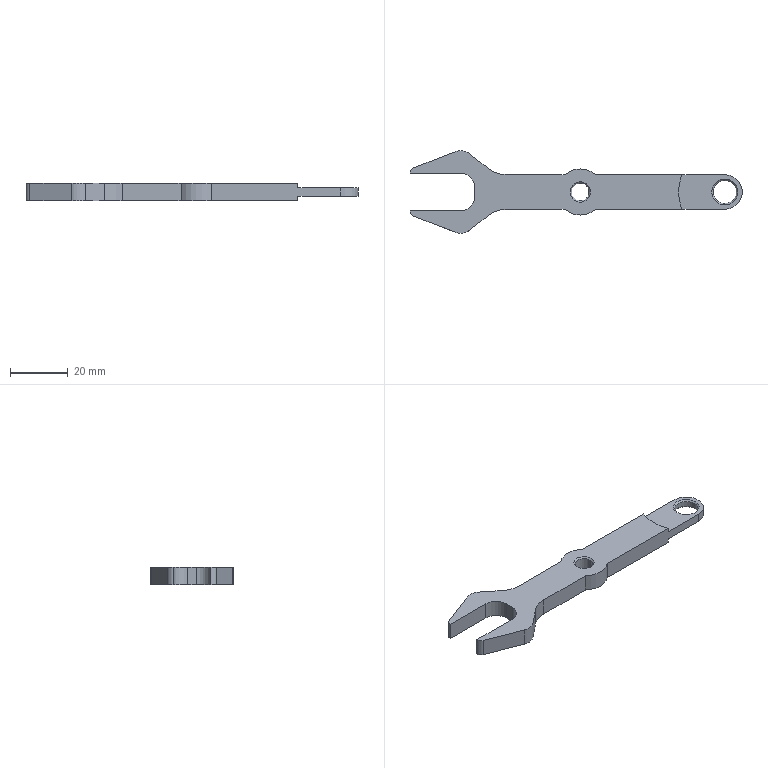Part | SolidWorks | features ICE 2, Chamfer 1, Extrusion 1, Fillet 1, MirrorPattern 1 | 1 solid | 41 faces | box 114.951 x 28.607 x 6 mm | volume 7418 mm3 | cylinder 18 | plane 15 | cone 8 | commonest cylinder face diameters 10 x4 32 x3 4 x2 6 x2 8 x2 16 x2
STEP:
#1=CARTESIAN_POINT('',(3.,0.,-2.5));
#2=VERTEX_POINT('',#1);
#3=CARTESIAN_POINT('',(-3.,0.,-2.5));
#4=VERTEX_POINT('',#3);
#5=CARTESIAN_POINT('',(0.,0.,-2.5));
#6=DIRECTION('',(0.,0.,-1.));
#7=DIRECTION('',(-1.,0.,0.));
#8=AXIS2_PLACEMENT_3D('',#5,#6,#7);
#9=CIRCLE('',#8,3.);
#10=EDGE_CURVE('',#2,#4,#9,.T.);
#11=ORIENTED_EDGE('',*,*,#10,.F.);
#12=CARTESIAN_POINT('',(3.5,0.,-3.));
#13=VERTEX_POINT('',#12);
#14=CARTESIAN_POINT('',(3.5,0.,-3.));
#15=DIRECTION('',(0.7071,0.,-0.7071));
#16=VECTOR('',#15,1000.);
#17=LINE('',#14,#16);
#18=EDGE_CURVE('',#2,#13,#17,.T.);
#19=ORIENTED_EDGE('',*,*,#18,.T.);
#20=CARTESIAN_POINT('',(-3.5,0.,-3.));
#21=VERTEX_POINT('',#20);
#22=CARTESIAN_POINT('',(0.,0.,-3.));
#23=DIRECTION('',(0.,0.,1.));
#24=DIRECTION('',(-1.,0.,0.));
#25=AXIS2_PLACEMENT_3D('',#22,#23,#24);
#26=CIRCLE('',#25,3.5);
#27=EDGE_CURVE('',#21,#13,#26,.T.);
#28=ORIENTED_EDGE('',*,*,#27,.F.);
#29=CARTESIAN_POINT('',(-3.5,0.,-3.));
#30=DIRECTION('',(-0.7071,0.,-0.7071));
#31=VECTOR('',#30,1000.);
#32=LINE('',#29,#31);
#33=EDGE_CURVE('',#4,#21,#32,.T.);
#34=ORIENTED_EDGE('',*,*,#33,.F.);
#35=EDGE_LOOP('',(#11,#19,#28,#34));
#36=FACE_OUTER_BOUND('',#35,.T.);
#37=CARTESIAN_POINT('',(0.,0.,-3.));
#38=DIRECTION('',(0.,0.,-1.));
#39=DIRECTION('',(-1.,0.,0.));
#40=AXIS2_PLACEMENT_3D('',#37,#38,#39);
#41=CONICAL_SURFACE('',#40,3.5,0.7854);
#42=ADVANCED_FACE('',(#36),#41,.F.);
#43=CARTESIAN_POINT('',(-3.,0.,2.5));
#44=VERTEX_POINT('',#43);
#45=CARTESIAN_POINT('',(3.,0.,2.5));
#46=VERTEX_POINT('',#45);
#47=CARTESIAN_POINT('',(0.,0.,2.5));
#48=DIRECTION('',(0.,0.,1.));
#49=DIRECTION('',(-1.,0.,0.));
#50=AXIS2_PLACEMENT_3D('',#47,#48,#49);
#51=CIRCLE('',#50,3.);
#52=EDGE_CURVE('',#44,#46,#51,.T.);
#53=ORIENTED_EDGE('',*,*,#52,.F.);
#54=CARTESIAN_POINT('',(-3.5,0.,3.));
#55=VERTEX_POINT('',#54);
#56=CARTESIAN_POINT('',(-3.,0.,2.5));
#57=DIRECTION('',(-0.7071,0.,0.7071));
#58=VECTOR('',#57,1000.);
#59=LINE('',#56,#58);
#60=EDGE_CURVE('',#44,#55,#59,.T.);
#61=ORIENTED_EDGE('',*,*,#60,.T.);
#62=CARTESIAN_POINT('',(3.5,0.,3.));
#63=VERTEX_POINT('',#62);
#64=CARTESIAN_POINT('',(0.,0.,3.));
#65=DIRECTION('',(0.,0.,-1.));
#66=DIRECTION('',(-1.,0.,0.));
#67=AXIS2_PLACEMENT_3D('',#64,#65,#66);
#68=CIRCLE('',#67,3.5);
#69=EDGE_CURVE('',#63,#55,#68,.T.);
#70=ORIENTED_EDGE('',*,*,#69,.F.);
#71=CARTESIAN_POINT('',(3.,0.,2.5));
#72=DIRECTION('',(0.7071,0.,0.7071));
#73=VECTOR('',#72,1000.);
#74=LINE('',#71,#73);
#75=EDGE_CURVE('',#46,#63,#74,.T.);
#76=ORIENTED_EDGE('',*,*,#75,.F.);
#77=EDGE_LOOP('',(#53,#61,#70,#76));
#78=FACE_OUTER_BOUND('',#77,.T.);
#79=CARTESIAN_POINT('',(0.,0.,2.5));
#80=DIRECTION('',(0.,0.,1.));
#81=DIRECTION('',(1.,0.,0.));
#82=AXIS2_PLACEMENT_3D('',#79,#80,#81);
#83=CONICAL_SURFACE('',#82,3.,0.7854);
#84=ADVANCED_FACE('',(#78),#83,.F.);
#85=CARTESIAN_POINT('',(46.,0.,1.));
#86=VERTEX_POINT('',#85);
#87=CARTESIAN_POINT('',(54.,0.,1.));
#88=VERTEX_POINT('',#87);
#89=CARTESIAN_POINT('',(50.,0.,1.));
#90=DIRECTION('',(0.,0.,1.));
#91=DIRECTION('',(1.,0.,0.));
#92=AXIS2_PLACEMENT_3D('',#89,#90,#91);
#93=CIRCLE('',#92,4.);
#94=EDGE_CURVE('',#86,#88,#93,.T.);
#95=ORIENTED_EDGE('',*,*,#94,.F.);
#96=CARTESIAN_POINT('',(45.5,0.,1.5));
#97=VERTEX_POINT('',#96);
#98=CARTESIAN_POINT('',(46.,0.,1.));
#99=DIRECTION('',(-0.7071,0.,0.7071));
#100=VECTOR('',#99,1000.);
#101=LINE('',#98,#100);
#102=EDGE_CURVE('',#86,#97,#101,.T.);
#103=ORIENTED_EDGE('',*,*,#102,.T.);
#104=CARTESIAN_POINT('',(54.5,0.,1.5));
#105=VERTEX_POINT('',#104);
#106=CARTESIAN_POINT('',(50.,0.,1.5));
#107=DIRECTION('',(0.,0.,-1.));
#108=DIRECTION('',(1.,0.,0.));
#109=AXIS2_PLACEMENT_3D('',#106,#107,#108);
#110=CIRCLE('',#109,4.5);
#111=EDGE_CURVE('',#105,#97,#110,.T.);
#112=ORIENTED_EDGE('',*,*,#111,.F.);
#113=CARTESIAN_POINT('',(54.,0.,1.));
#114=DIRECTION('',(0.7071,0.,0.7071));
#115=VECTOR('',#114,1000.);
#116=LINE('',#113,#115);
#117=EDGE_CURVE('',#88,#105,#116,.T.);
#118=ORIENTED_EDGE('',*,*,#117,.F.);
#119=EDGE_LOOP('',(#95,#103,#112,#118));
#120=FACE_OUTER_BOUND('',#119,.T.);
#121=CARTESIAN_POINT('',(50.,0.,1.));
#122=DIRECTION('',(0.,0.,1.));
#123=DIRECTION('',(1.,0.,0.));
#124=AXIS2_PLACEMENT_3D('',#121,#122,#123);
#125=CONICAL_SURFACE('',#124,4.,0.7854);
#126=ADVANCED_FACE('',(#120),#125,.F.);
#127=CARTESIAN_POINT('',(54.,0.,-1.));
#128=VERTEX_POINT('',#127);
#129=CARTESIAN_POINT('',(46.,0.,-1.));
#130=VERTEX_POINT('',#129);
#131=CARTESIAN_POINT('',(50.,0.,-1.));
#132=DIRECTION('',(0.,0.,-1.));
#133=DIRECTION('',(-1.,0.,0.));
#134=AXIS2_PLACEMENT_3D('',#131,#132,#133);
#135=CIRCLE('',#134,4.);
#136=EDGE_CURVE('',#128,#130,#135,.T.);
#137=ORIENTED_EDGE('',*,*,#136,.F.);
#138=CARTESIAN_POINT('',(54.5,0.,-1.5));
#139=VERTEX_POINT('',#138);
#140=CARTESIAN_POINT('',(54.,0.,-1.));
#141=DIRECTION('',(0.7071,0.,-0.7071));
#142=VECTOR('',#141,1000.);
#143=LINE('',#140,#142);
#144=EDGE_CURVE('',#128,#139,#143,.T.);
#145=ORIENTED_EDGE('',*,*,#144,.T.);
#146=CARTESIAN_POINT('',(45.5,0.,-1.5));
#147=VERTEX_POINT('',#146);
#148=CARTESIAN_POINT('',(50.,0.,-1.5));
#149=DIRECTION('',(0.,0.,1.));
#150=DIRECTION('',(-1.,0.,0.));
#151=AXIS2_PLACEMENT_3D('',#148,#149,#150);
#152=CIRCLE('',#151,4.5);
#153=EDGE_CURVE('',#147,#139,#152,.T.);
#154=ORIENTED_EDGE('',*,*,#153,.F.);
#155=CARTESIAN_POINT('',(46.,0.,-1.));
#156=DIRECTION('',(-0.7071,0.,-0.7071));
#157=VECTOR('',#156,1000.);
#158=LINE('',#155,#157);
#159=EDGE_CURVE('',#130,#147,#158,.T.);
#160=ORIENTED_EDGE('',*,*,#159,.F.);
#161=EDGE_LOOP('',(#137,#145,#154,#160));
#162=FACE_OUTER_BOUND('',#161,.T.);
#163=CARTESIAN_POINT('',(50.,0.,-1.));
#164=DIRECTION('',(0.,0.,-1.));
#165=DIRECTION('',(-1.,0.,0.));
#166=AXIS2_PLACEMENT_3D('',#163,#164,#165);
#167=CONICAL_SURFACE('',#166,4.,0.7854);
#168=ADVANCED_FACE('',(#162),#167,.F.);
#169=ORIENTED_EDGE('',*,*,#10,.T.);
#170=CARTESIAN_POINT('',(-3.,0.,-3.));
#171=DIRECTION('',(0.,0.,1.));
#172=VECTOR('',#171,1000.);
#173=LINE('',#170,#172);
#174=EDGE_CURVE('',#4,#44,#173,.T.);
#175=ORIENTED_EDGE('',*,*,#174,.T.);
#176=ORIENTED_EDGE('',*,*,#52,.T.);
#177=CARTESIAN_POINT('',(3.,0.,-3.));
#178=DIRECTION('',(0.,0.,1.));
#179=VECTOR('',#178,1000.);
#180=LINE('',#177,#179);
#181=EDGE_CURVE('',#2,#46,#180,.T.);
#182=ORIENTED_EDGE('',*,*,#181,.F.);
#183=EDGE_LOOP('',(#169,#175,#176,#182));
#184=FACE_OUTER_BOUND('',#183,.T.);
#185=CARTESIAN_POINT('',(0.,0.,-3.));
#186=DIRECTION('',(0.,0.,1.));
#187=DIRECTION('',(1.,0.,0.));
#188=AXIS2_PLACEMENT_3D('',#185,#186,#187);
#189=CYLINDRICAL_SURFACE('',#188,3.);
#190=ADVANCED_FACE('',(#184),#189,.F.);
#191=ORIENTED_EDGE('',*,*,#136,.T.);
#192=CARTESIAN_POINT('',(46.,0.,-3.));
#193=DIRECTION('',(0.,0.,1.));
#194=VECTOR('',#193,1000.);
#195=LINE('',#192,#194);
#196=EDGE_CURVE('',#130,#86,#195,.T.);
#197=ORIENTED_EDGE('',*,*,#196,.T.);
#198=ORIENTED_EDGE('',*,*,#94,.T.);
#199=CARTESIAN_POINT('',(54.,0.,-3.));
#200=DIRECTION('',(0.,0.,1.));
#201=VECTOR('',#200,1000.);
#202=LINE('',#199,#201);
#203=EDGE_CURVE('',#128,#88,#202,.T.);
#204=ORIENTED_EDGE('',*,*,#203,.F.);
#205=EDGE_LOOP('',(#191,#197,#198,#204));
#206=FACE_OUTER_BOUND('',#205,.T.);
#207=CARTESIAN_POINT('',(50.,0.,-3.));
#208=DIRECTION('',(0.,0.,1.));
#209=DIRECTION('',(1.,0.,0.));
#210=AXIS2_PLACEMENT_3D('',#207,#208,#209);
#211=CYLINDRICAL_SURFACE('',#210,4.);
#212=ADVANCED_FACE('',(#206),#211,.F.);
#213=CARTESIAN_POINT('',(35.168,6.,-1.5));
#214=VERTEX_POINT('',#213);
#215=CARTESIAN_POINT('',(34.,0.,-1.5));
#216=VERTEX_POINT('',#215);
#217=CARTESIAN_POINT('',(50.,0.,-1.5));
#218=DIRECTION('',(0.,0.,1.));
#219=DIRECTION('',(1.,0.,0.));
#220=AXIS2_PLACEMENT_3D('',#217,#218,#219);
#221=CIRCLE('',#220,16.);
#222=EDGE_CURVE('',#214,#216,#221,.T.);
#223=ORIENTED_EDGE('',*,*,#222,.T.);
#224=CARTESIAN_POINT('',(34.,0.,-3.));
#225=VERTEX_POINT('',#224);
#226=CARTESIAN_POINT('',(34.,0.,-1.5));
#227=DIRECTION('',(0.,0.,-1.));
#228=VECTOR('',#227,1000.);
#229=LINE('',#226,#228);
#230=EDGE_CURVE('',#216,#225,#229,.T.);
#231=ORIENTED_EDGE('',*,*,#230,.T.);
#232=CARTESIAN_POINT('',(35.168,6.,-3.));
#233=VERTEX_POINT('',#232);
#234=CARTESIAN_POINT('',(50.,0.,-3.));
#235=DIRECTION('',(0.,0.,1.));
#236=DIRECTION('',(1.,0.,0.));
#237=AXIS2_PLACEMENT_3D('',#234,#235,#236);
#238=CIRCLE('',#237,16.);
#239=EDGE_CURVE('',#233,#225,#238,.T.);
#240=ORIENTED_EDGE('',*,*,#239,.F.);
#241=CARTESIAN_POINT('',(35.168,6.,-1.5));
#242=DIRECTION('',(0.,0.,1.));
#243=VECTOR('',#242,1000.);
#244=LINE('',#241,#243);
#245=EDGE_CURVE('',#233,#214,#244,.T.);
#246=ORIENTED_EDGE('',*,*,#245,.T.);
#247=EDGE_LOOP('',(#223,#231,#240,#246));
#248=FACE_OUTER_BOUND('',#247,.T.);
#249=CARTESIAN_POINT('',(50.,0.,-1.5));
#250=DIRECTION('',(0.,0.,-1.));
#251=DIRECTION('',(-1.,0.,0.));
#252=AXIS2_PLACEMENT_3D('',#249,#250,#251);
#253=CYLINDRICAL_SURFACE('',#252,16.);
#254=ADVANCED_FACE('',(#248),#253,.F.);
#255=CARTESIAN_POINT('',(50.,6.,-1.5));
#256=VERTEX_POINT('',#255);
#257=CARTESIAN_POINT('',(50.,-6.,-1.5));
#258=VERTEX_POINT('',#257);
#259=CARTESIAN_POINT('',(50.,0.,-1.5));
#260=DIRECTION('',(0.,0.,-1.));
#261=DIRECTION('',(-1.,0.,0.));
#262=AXIS2_PLACEMENT_3D('',#259,#260,#261);
#263=CIRCLE('',#262,6.);
#264=EDGE_CURVE('',#256,#258,#263,.T.);
#265=ORIENTED_EDGE('',*,*,#264,.F.);
#266=CARTESIAN_POINT('',(50.,6.,1.5));
#267=VERTEX_POINT('',#266);
#268=CARTESIAN_POINT('',(50.,6.,3.));
#269=DIRECTION('',(0.,0.,-1.));
#270=VECTOR('',#269,1000.);
#271=LINE('',#268,#270);
#272=EDGE_CURVE('',#267,#256,#271,.T.);
#273=ORIENTED_EDGE('',*,*,#272,.F.);
#274=CARTESIAN_POINT('',(50.,-6.,1.5));
#275=VERTEX_POINT('',#274);
#276=CARTESIAN_POINT('',(50.,0.,1.5));
#277=DIRECTION('',(0.,0.,1.));
#278=DIRECTION('',(1.,0.,0.));
#279=AXIS2_PLACEMENT_3D('',#276,#277,#278);
#280=CIRCLE('',#279,6.);
#281=EDGE_CURVE('',#275,#267,#280,.T.);
#282=ORIENTED_EDGE('',*,*,#281,.F.);
#283=CARTESIAN_POINT('',(50.,-6.,3.));
#284=DIRECTION('',(0.,0.,-1.));
#285=VECTOR('',#284,1000.);
#286=LINE('',#283,#285);
#287=EDGE_CURVE('',#275,#258,#286,.T.);
#288=ORIENTED_EDGE('',*,*,#287,.T.);
#289=EDGE_LOOP('',(#265,#273,#282,#288));
#290=FACE_OUTER_BOUND('',#289,.T.);
#291=CARTESIAN_POINT('',(50.,0.,3.));
#292=DIRECTION('',(0.,0.,-1.));
#293=DIRECTION('',(-1.,0.,0.));
#294=AXIS2_PLACEMENT_3D('',#291,#292,#293);
#295=CYLINDRICAL_SURFACE('',#294,6.);
#296=ADVANCED_FACE('',(#290),#295,.T.);
#297=CARTESIAN_POINT('',(35.168,-6.,-1.5));
#298=VERTEX_POINT('',#297);
#299=CARTESIAN_POINT('',(35.168,-6.,-3.));
#300=VERTEX_POINT('',#299);
#301=CARTESIAN_POINT('',(35.168,-6.,-1.5));
#302=DIRECTION('',(0.,0.,-1.));
#303=VECTOR('',#302,1000.);
#304=LINE('',#301,#303);
#305=EDGE_CURVE('',#298,#300,#304,.T.);
#306=ORIENTED_EDGE('',*,*,#305,.F.);
#307=CARTESIAN_POINT('',(50.,-6.,-1.5));
#308=DIRECTION('',(-1.,0.,0.));
#309=VECTOR('',#308,1000.);
#310=LINE('',#307,#309);
#311=EDGE_CURVE('',#258,#298,#310,.T.);
#312=ORIENTED_EDGE('',*,*,#311,.F.);
#313=ORIENTED_EDGE('',*,*,#287,.F.);
#314=CARTESIAN_POINT('',(35.168,-6.,1.5));
#315=VERTEX_POINT('',#314);
#316=CARTESIAN_POINT('',(50.,-6.,1.5));
#317=DIRECTION('',(1.,0.,0.));
#318=VECTOR('',#317,1000.);
#319=LINE('',#316,#318);
#320=EDGE_CURVE('',#315,#275,#319,.T.);
#321=ORIENTED_EDGE('',*,*,#320,.F.);
#322=CARTESIAN_POINT('',(35.168,-6.,3.));
#323=VERTEX_POINT('',#322);
#324=CARTESIAN_POINT('',(35.168,-6.,1.5));
#325=DIRECTION('',(0.,0.,1.));
#326=VECTOR('',#325,1000.);
#327=LINE('',#324,#326);
#328=EDGE_CURVE('',#315,#323,#327,.T.);
#329=ORIENTED_EDGE('',*,*,#328,.T.);
#330=CARTESIAN_POINT('',(5.292,-6.,3.));
#331=VERTEX_POINT('',#330);
#332=CARTESIAN_POINT('',(50.,-6.,3.));
#333=DIRECTION('',(1.,0.,0.));
#334=VECTOR('',#333,1000.);
#335=LINE('',#332,#334);
#336=EDGE_CURVE('',#331,#323,#335,.T.);
#337=ORIENTED_EDGE('',*,*,#336,.F.);
#338=CARTESIAN_POINT('',(5.292,-6.,-3.));
#339=VERTEX_POINT('',#338);
#340=CARTESIAN_POINT('',(5.292,-6.,3.));
#341=DIRECTION('',(0.,0.,-1.));
#342=VECTOR('',#341,1000.);
#343=LINE('',#340,#342);
#344=EDGE_CURVE('',#331,#339,#343,.T.);
#345=ORIENTED_EDGE('',*,*,#344,.T.);
#346=CARTESIAN_POINT('',(50.,-6.,-3.));
#347=DIRECTION('',(1.,0.,0.));
#348=VECTOR('',#347,1000.);
#349=LINE('',#346,#348);
#350=EDGE_CURVE('',#339,#300,#349,.T.);
#351=ORIENTED_EDGE('',*,*,#350,.T.);
#352=EDGE_LOOP('',(#306,#312,#313,#321,#329,#337,#345,#351));
#353=FACE_OUTER_BOUND('',#352,.T.);
#354=CARTESIAN_POINT('',(50.,-6.,3.));
#355=DIRECTION('',(0.,1.,0.));
#356=DIRECTION('',(0.,0.,1.));
#357=AXIS2_PLACEMENT_3D('',#354,#355,#356);
#358=PLANE('',#357);
#359=ADVANCED_FACE('',(#353),#358,.F.);
#360=ORIENTED_EDGE('',*,*,#245,.F.);
#361=CARTESIAN_POINT('',(5.292,6.,-3.));
#362=VERTEX_POINT('',#361);
#363=CARTESIAN_POINT('',(50.,6.,-3.));
#364=DIRECTION('',(-1.,0.,0.));
#365=VECTOR('',#364,1000.);
#366=LINE('',#363,#365);
#367=EDGE_CURVE('',#233,#362,#366,.T.);
#368=ORIENTED_EDGE('',*,*,#367,.T.);
#369=CARTESIAN_POINT('',(5.292,6.,3.));
#370=VERTEX_POINT('',#369);
#371=CARTESIAN_POINT('',(5.292,6.,3.));
#372=DIRECTION('',(0.,0.,-1.));
#373=VECTOR('',#372,1000.);
#374=LINE('',#371,#373);
#375=EDGE_CURVE('',#370,#362,#374,.T.);
#376=ORIENTED_EDGE('',*,*,#375,.F.);
#377=CARTESIAN_POINT('',(35.168,6.,3.));
#378=VERTEX_POINT('',#377);
#379=CARTESIAN_POINT('',(50.,6.,3.));
#380=DIRECTION('',(-1.,0.,0.));
#381=VECTOR('',#380,1000.);
#382=LINE('',#379,#381);
#383=EDGE_CURVE('',#378,#370,#382,.T.);
#384=ORIENTED_EDGE('',*,*,#383,.F.);
#385=CARTESIAN_POINT('',(35.168,6.,1.5));
#386=VERTEX_POINT('',#385);
#387=CARTESIAN_POINT('',(35.168,6.,1.5));
#388=DIRECTION('',(0.,0.,-1.));
#389=VECTOR('',#388,1000.);
#390=LINE('',#387,#389);
#391=EDGE_CURVE('',#378,#386,#390,.T.);
#392=ORIENTED_EDGE('',*,*,#391,.T.);
#393=CARTESIAN_POINT('',(50.,6.,1.5));
#394=DIRECTION('',(-1.,0.,0.));
#395=VECTOR('',#394,1000.);
#396=LINE('',#393,#395);
#397=EDGE_CURVE('',#267,#386,#396,.T.);
#398=ORIENTED_EDGE('',*,*,#397,.F.);
#399=ORIENTED_EDGE('',*,*,#272,.T.);
#400=CARTESIAN_POINT('',(50.,6.,-1.5));
#401=DIRECTION('',(1.,0.,0.));
#402=VECTOR('',#401,1000.);
#403=LINE('',#400,#402);
#404=EDGE_CURVE('',#214,#256,#403,.T.);
#405=ORIENTED_EDGE('',*,*,#404,.F.);
#406=EDGE_LOOP('',(#360,#368,#376,#384,#392,#398,#399,#405));
#407=FACE_OUTER_BOUND('',#406,.T.);
#408=CARTESIAN_POINT('',(50.,6.,3.));
#409=DIRECTION('',(0.,-1.,0.));
#410=DIRECTION('',(0.,0.,-1.));
#411=AXIS2_PLACEMENT_3D('',#408,#409,#410);
#412=PLANE('',#411);
#413=ADVANCED_FACE('',(#407),#412,.F.);
#414=CARTESIAN_POINT('',(-43.172,-13.967,-3.));
#415=VERTEX_POINT('',#414);
#416=CARTESIAN_POINT('',(-38.258,-13.217,-3.));
#417=VERTEX_POINT('',#416);
#418=CARTESIAN_POINT('',(-41.37,-9.303,-3.));
#419=DIRECTION('',(0.,0.,1.));
#420=DIRECTION('',(-1.,0.,0.));
#421=AXIS2_PLACEMENT_3D('',#418,#419,#420);
#422=CIRCLE('',#421,5.);
#423=EDGE_CURVE('',#415,#417,#422,.T.);
#424=ORIENTED_EDGE('',*,*,#423,.T.);
#425=CARTESIAN_POINT('',(-38.258,-13.217,3.));
#426=VERTEX_POINT('',#425);
#427=CARTESIAN_POINT('',(-38.258,-13.217,3.));
#428=DIRECTION('',(0.,0.,-1.));
#429=VECTOR('',#428,1000.);
#430=LINE('',#427,#429);
#431=EDGE_CURVE('',#426,#417,#430,.T.);
#432=ORIENTED_EDGE('',*,*,#431,.F.);
#433=CARTESIAN_POINT('',(-43.172,-13.967,3.));
#434=VERTEX_POINT('',#433);
#435=CARTESIAN_POINT('',(-41.37,-9.303,3.));
#436=DIRECTION('',(0.,0.,1.));
#437=DIRECTION('',(-1.,0.,0.));
#438=AXIS2_PLACEMENT_3D('',#435,#436,#437);
#439=CIRCLE('',#438,5.);
#440=EDGE_CURVE('',#434,#426,#439,.T.);
#441=ORIENTED_EDGE('',*,*,#440,.F.);
#442=CARTESIAN_POINT('',(-43.172,-13.967,3.));
#443=DIRECTION('',(0.,0.,-1.));
#444=VECTOR('',#443,1000.);
#445=LINE('',#442,#444);
#446=EDGE_CURVE('',#434,#415,#445,.T.);
#447=ORIENTED_EDGE('',*,*,#446,.T.);
#448=EDGE_LOOP('',(#424,#432,#441,#447));
#449=FACE_OUTER_BOUND('',#448,.T.);
#450=CARTESIAN_POINT('',(-41.37,-9.303,3.));
#451=DIRECTION('',(0.,0.,-1.));
#452=DIRECTION('',(-1.,0.,0.));
#453=AXIS2_PLACEMENT_3D('',#450,#451,#452);
#454=CYLINDRICAL_SURFACE('',#453,5.);
#455=ADVANCED_FACE('',(#449),#454,.T.);
#456=CARTESIAN_POINT('',(-31.918,-8.174,-3.));
#457=VERTEX_POINT('',#456);
#458=CARTESIAN_POINT('',(-29.185,-6.,-3.));
#459=DIRECTION('',(0.7826,0.6225,0.));
#460=VECTOR('',#459,1000.);
#461=LINE('',#458,#460);
#462=EDGE_CURVE('',#417,#457,#461,.T.);
#463=ORIENTED_EDGE('',*,*,#462,.T.);
#464=CARTESIAN_POINT('',(-31.918,-8.174,3.));
#465=VERTEX_POINT('',#464);
#466=CARTESIAN_POINT('',(-31.918,-8.174,3.));
#467=DIRECTION('',(0.,0.,1.));
#468=VECTOR('',#467,1000.);
#469=LINE('',#466,#468);
#470=EDGE_CURVE('',#457,#465,#469,.T.);
#471=ORIENTED_EDGE('',*,*,#470,.T.);
#472=CARTESIAN_POINT('',(-29.185,-6.,3.));
#473=DIRECTION('',(0.7826,0.6225,0.));
#474=VECTOR('',#473,1000.);
#475=LINE('',#472,#474);
#476=EDGE_CURVE('',#426,#465,#475,.T.);
#477=ORIENTED_EDGE('',*,*,#476,.F.);
#478=ORIENTED_EDGE('',*,*,#431,.T.);
#479=EDGE_LOOP('',(#463,#471,#477,#478));
#480=FACE_OUTER_BOUND('',#479,.T.);
#481=CARTESIAN_POINT('',(-29.185,-6.,3.));
#482=DIRECTION('',(-0.6225,0.7826,0.));
#483=DIRECTION('',(-0.7826,-0.6225,0.));
#484=AXIS2_PLACEMENT_3D('',#481,#482,#483);
#485=PLANE('',#484);
#486=ADVANCED_FACE('',(#480),#485,.F.);
#487=CARTESIAN_POINT('',(-25.693,-6.,3.));
#488=VERTEX_POINT('',#487);
#489=CARTESIAN_POINT('',(-5.292,-6.,3.));
#490=VERTEX_POINT('',#489);
#491=CARTESIAN_POINT('',(-5.292,-6.,3.));
#492=DIRECTION('',(1.,0.,0.));
#493=VECTOR('',#492,1000.);
#494=LINE('',#491,#493);
#495=EDGE_CURVE('',#488,#490,#494,.T.);
#496=ORIENTED_EDGE('',*,*,#495,.F.);
#497=CARTESIAN_POINT('',(-25.693,-6.,-3.));
#498=VERTEX_POINT('',#497);
#499=CARTESIAN_POINT('',(-25.693,-6.,-3.));
#500=DIRECTION('',(0.,0.,-1.));
#501=VECTOR('',#500,1000.);
#502=LINE('',#499,#501);
#503=EDGE_CURVE('',#488,#498,#502,.T.);
#504=ORIENTED_EDGE('',*,*,#503,.T.);
#505=CARTESIAN_POINT('',(-5.292,-6.,-3.));
#506=VERTEX_POINT('',#505);
#507=CARTESIAN_POINT('',(-5.292,-6.,-3.));
#508=DIRECTION('',(1.,0.,0.));
#509=VECTOR('',#508,1000.);
#510=LINE('',#507,#509);
#511=EDGE_CURVE('',#498,#506,#510,.T.);
#512=ORIENTED_EDGE('',*,*,#511,.T.);
#513=CARTESIAN_POINT('',(-5.292,-6.,3.));
#514=DIRECTION('',(0.,0.,-1.));
#515=VECTOR('',#514,1000.);
#516=LINE('',#513,#515);
#517=EDGE_CURVE('',#490,#506,#516,.T.);
#518=ORIENTED_EDGE('',*,*,#517,.F.);
#519=EDGE_LOOP('',(#496,#504,#512,#518));
#520=FACE_OUTER_BOUND('',#519,.T.);
#521=CARTESIAN_POINT('',(-5.292,-6.,3.));
#522=DIRECTION('',(0.,1.,0.));
#523=DIRECTION('',(-1.,0.,0.));
#524=AXIS2_PLACEMENT_3D('',#521,#522,#523);
#525=PLANE('',#524);
#526=ADVANCED_FACE('',(#520),#525,.F.);
#527=CARTESIAN_POINT('',(0.,0.,-3.));
#528=DIRECTION('',(0.,0.,1.));
#529=DIRECTION('',(-1.,0.,0.));
#530=AXIS2_PLACEMENT_3D('',#527,#528,#529);
#531=CIRCLE('',#530,8.);
#532=EDGE_CURVE('',#506,#339,#531,.T.);
#533=ORIENTED_EDGE('',*,*,#532,.T.);
#534=ORIENTED_EDGE('',*,*,#344,.F.);
#535=CARTESIAN_POINT('',(0.,0.,3.));
#536=DIRECTION('',(0.,0.,1.));
#537=DIRECTION('',(-1.,0.,0.));
#538=AXIS2_PLACEMENT_3D('',#535,#536,#537);
#539=CIRCLE('',#538,8.);
#540=EDGE_CURVE('',#490,#331,#539,.T.);
#541=ORIENTED_EDGE('',*,*,#540,.F.);
#542=ORIENTED_EDGE('',*,*,#517,.T.);
#543=EDGE_LOOP('',(#533,#534,#541,#542));
#544=FACE_OUTER_BOUND('',#543,.T.);
#545=CARTESIAN_POINT('',(0.,0.,3.));
#546=DIRECTION('',(0.,0.,-1.));
#547=DIRECTION('',(-1.,0.,0.));
#548=AXIS2_PLACEMENT_3D('',#545,#546,#547);
#549=CYLINDRICAL_SURFACE('',#548,8.);
#550=ADVANCED_FACE('',(#544),#549,.T.);
#551=CARTESIAN_POINT('',(-5.292,6.,-3.));
#552=VERTEX_POINT('',#551);
#553=CARTESIAN_POINT('',(0.,0.,-3.));
#554=DIRECTION('',(0.,0.,1.));
#555=DIRECTION('',(1.,0.,0.));
#556=AXIS2_PLACEMENT_3D('',#553,#554,#555);
#557=CIRCLE('',#556,8.);
#558=EDGE_CURVE('',#362,#552,#557,.T.);
#559=ORIENTED_EDGE('',*,*,#558,.T.);
#560=CARTESIAN_POINT('',(-5.292,6.,3.));
#561=VERTEX_POINT('',#560);
#562=CARTESIAN_POINT('',(-5.292,6.,3.));
#563=DIRECTION('',(0.,0.,-1.));
#564=VECTOR('',#563,1000.);
#565=LINE('',#562,#564);
#566=EDGE_CURVE('',#561,#552,#565,.T.);
#567=ORIENTED_EDGE('',*,*,#566,.F.);
#568=CARTESIAN_POINT('',(0.,0.,3.));
#569=DIRECTION('',(0.,0.,1.));
#570=DIRECTION('',(1.,0.,0.));
#571=AXIS2_PLACEMENT_3D('',#568,#569,#570);
#572=CIRCLE('',#571,8.);
#573=EDGE_CURVE('',#370,#561,#572,.T.);
#574=ORIENTED_EDGE('',*,*,#573,.F.);
#575=ORIENTED_EDGE('',*,*,#375,.T.);
#576=EDGE_LOOP('',(#559,#567,#574,#575));
#577=FACE_OUTER_BOUND('',#576,.T.);
#578=CARTESIAN_POINT('',(0.,0.,3.));
#579=DIRECTION('',(0.,0.,-1.));
#580=DIRECTION('',(-1.,0.,0.));
#581=AXIS2_PLACEMENT_3D('',#578,#579,#580);
#582=CYLINDRICAL_SURFACE('',#581,8.);
#583=ADVANCED_FACE('',(#577),#582,.T.);
#584=CARTESIAN_POINT('',(-25.693,6.,-3.));
#585=VERTEX_POINT('',#584);
#586=CARTESIAN_POINT('',(-5.292,6.,-3.));
#587=DIRECTION('',(-1.,0.,0.));
#588=VECTOR('',#587,1000.);
#589=LINE('',#586,#588);
#590=EDGE_CURVE('',#552,#585,#589,.T.);
#591=ORIENTED_EDGE('',*,*,#590,.T.);
#592=CARTESIAN_POINT('',(-25.693,6.,3.));
#593=VERTEX_POINT('',#592);
#594=CARTESIAN_POINT('',(-25.693,6.,3.));
#595=DIRECTION('',(0.,0.,1.));
#596=VECTOR('',#595,1000.);
#597=LINE('',#594,#596);
#598=EDGE_CURVE('',#585,#593,#597,.T.);
#599=ORIENTED_EDGE('',*,*,#598,.T.);
#600=CARTESIAN_POINT('',(-5.292,6.,3.));
#601=DIRECTION('',(-1.,0.,0.));
#602=VECTOR('',#601,1000.);
#603=LINE('',#600,#602);
#604=EDGE_CURVE('',#561,#593,#603,.T.);
#605=ORIENTED_EDGE('',*,*,#604,.F.);
#606=ORIENTED_EDGE('',*,*,#566,.T.);
#607=EDGE_LOOP('',(#591,#599,#605,#606));
#608=FACE_OUTER_BOUND('',#607,.T.);
#609=CARTESIAN_POINT('',(-5.292,6.,3.));
#610=DIRECTION('',(0.,-1.,0.));
#611=DIRECTION('',(1.,0.,0.));
#612=AXIS2_PLACEMENT_3D('',#609,#610,#611);
#613=PLANE('',#612);
#614=ADVANCED_FACE('',(#608),#613,.F.);
#615=CARTESIAN_POINT('',(-31.918,8.174,3.));
#616=VERTEX_POINT('',#615);
#617=CARTESIAN_POINT('',(-38.258,13.217,3.));
#618=VERTEX_POINT('',#617);
#619=CARTESIAN_POINT('',(-29.185,6.,3.));
#620=DIRECTION('',(-0.7826,0.6225,0.));
#621=VECTOR('',#620,1000.);
#622=LINE('',#619,#621);
#623=EDGE_CURVE('',#616,#618,#622,.T.);
#624=ORIENTED_EDGE('',*,*,#623,.F.);
#625=CARTESIAN_POINT('',(-31.918,8.174,-3.));
#626=VERTEX_POINT('',#625);
#627=CARTESIAN_POINT('',(-31.918,8.174,-3.));
#628=DIRECTION('',(0.,0.,-1.));
#629=VECTOR('',#628,1000.);
#630=LINE('',#627,#629);
#631=EDGE_CURVE('',#616,#626,#630,.T.);
#632=ORIENTED_EDGE('',*,*,#631,.T.);
#633=CARTESIAN_POINT('',(-38.258,13.217,-3.));
#634=VERTEX_POINT('',#633);
#635=CARTESIAN_POINT('',(-29.185,6.,-3.));
#636=DIRECTION('',(-0.7826,0.6225,0.));
#637=VECTOR('',#636,1000.);
#638=LINE('',#635,#637);
#639=EDGE_CURVE('',#626,#634,#638,.T.);
#640=ORIENTED_EDGE('',*,*,#639,.T.);
#641=CARTESIAN_POINT('',(-38.258,13.217,3.));
#642=DIRECTION('',(0.,0.,-1.));
#643=VECTOR('',#642,1000.);
#644=LINE('',#641,#643);
#645=EDGE_CURVE('',#618,#634,#644,.T.);
#646=ORIENTED_EDGE('',*,*,#645,.F.);
#647=EDGE_LOOP('',(#624,#632,#640,#646));
#648=FACE_OUTER_BOUND('',#647,.T.);
#649=CARTESIAN_POINT('',(-29.185,6.,3.));
#650=DIRECTION('',(-0.6225,-0.7826,0.));
#651=DIRECTION('',(0.7826,-0.6225,0.));
#652=AXIS2_PLACEMENT_3D('',#649,#650,#651);
#653=PLANE('',#652);
#654=ADVANCED_FACE('',(#648),#653,.F.);
#655=CARTESIAN_POINT('',(-43.172,13.967,-3.));
#656=VERTEX_POINT('',#655);
#657=CARTESIAN_POINT('',(-41.37,9.303,-3.));
#658=DIRECTION('',(0.,0.,1.));
#659=DIRECTION('',(1.,0.,0.));
#660=AXIS2_PLACEMENT_3D('',#657,#658,#659);
#661=CIRCLE('',#660,5.);
#662=EDGE_CURVE('',#634,#656,#661,.T.);
#663=ORIENTED_EDGE('',*,*,#662,.T.);
#664=CARTESIAN_POINT('',(-43.172,13.967,3.));
#665=VERTEX_POINT('',#664);
#666=CARTESIAN_POINT('',(-43.172,13.967,3.));
#667=DIRECTION('',(0.,0.,-1.));
#668=VECTOR('',#667,1000.);
#669=LINE('',#666,#668);
#670=EDGE_CURVE('',#665,#656,#669,.T.);
#671=ORIENTED_EDGE('',*,*,#670,.F.);
#672=CARTESIAN_POINT('',(-41.37,9.303,3.));
#673=DIRECTION('',(0.,0.,1.));
#674=DIRECTION('',(1.,0.,0.));
#675=AXIS2_PLACEMENT_3D('',#672,#673,#674);
#676=CIRCLE('',#675,5.);
#677=EDGE_CURVE('',#618,#665,#676,.T.);
#678=ORIENTED_EDGE('',*,*,#677,.F.);
#679=ORIENTED_EDGE('',*,*,#645,.T.);
#680=EDGE_LOOP('',(#663,#671,#678,#679));
#681=FACE_OUTER_BOUND('',#680,.T.);
#682=CARTESIAN_POINT('',(-41.37,9.303,3.));
#683=DIRECTION('',(0.,0.,-1.));
#684=DIRECTION('',(-1.,0.,0.));
#685=AXIS2_PLACEMENT_3D('',#682,#683,#684);
#686=CYLINDRICAL_SURFACE('',#685,5.);
#687=ADVANCED_FACE('',(#681),#686,.T.);
#688=CARTESIAN_POINT('',(-57.671,8.366,-3.));
#689=VERTEX_POINT('',#688);
#690=CARTESIAN_POINT('',(-43.172,13.967,-3.));
#691=DIRECTION('',(-0.9328,-0.3604,0.));
#692=VECTOR('',#691,1000.);
#693=LINE('',#690,#692);
#694=EDGE_CURVE('',#656,#689,#693,.T.);
#695=ORIENTED_EDGE('',*,*,#694,.T.);
#696=CARTESIAN_POINT('',(-57.671,8.366,3.));
#697=VERTEX_POINT('',#696);
#698=CARTESIAN_POINT('',(-57.671,8.366,3.));
#699=DIRECTION('',(0.,0.,-1.));
#700=VECTOR('',#699,1000.);
#701=LINE('',#698,#700);
#702=EDGE_CURVE('',#697,#689,#701,.T.);
#703=ORIENTED_EDGE('',*,*,#702,.F.);
#704=CARTESIAN_POINT('',(-43.172,13.967,3.));
#705=DIRECTION('',(-0.9328,-0.3604,0.));
#706=VECTOR('',#705,1000.);
#707=LINE('',#704,#706);
#708=EDGE_CURVE('',#665,#697,#707,.T.);
#709=ORIENTED_EDGE('',*,*,#708,.F.);
#710=ORIENTED_EDGE('',*,*,#670,.T.);
#711=EDGE_LOOP('',(#695,#703,#709,#710));
#712=FACE_OUTER_BOUND('',#711,.T.);
#713=CARTESIAN_POINT('',(-43.172,13.967,3.));
#714=DIRECTION('',(0.3604,-0.9328,0.));
#715=DIRECTION('',(0.9328,0.3604,0.));
#716=AXIS2_PLACEMENT_3D('',#713,#714,#715);
#717=PLANE('',#716);
#718=ADVANCED_FACE('',(#712),#717,.F.);
#719=CARTESIAN_POINT('',(-58.951,6.5,-3.));
#720=VERTEX_POINT('',#719);
#721=CARTESIAN_POINT('',(-56.951,6.5,-3.));
#722=DIRECTION('',(0.,0.,1.));
#723=DIRECTION('',(-1.,0.,0.));
#724=AXIS2_PLACEMENT_3D('',#721,#722,#723);
#725=CIRCLE('',#724,2.);
#726=EDGE_CURVE('',#689,#720,#725,.T.);
#727=ORIENTED_EDGE('',*,*,#726,.T.);
#728=CARTESIAN_POINT('',(-58.951,6.5,3.));
#729=VERTEX_POINT('',#728);
#730=CARTESIAN_POINT('',(-58.951,6.5,3.));
#731=DIRECTION('',(0.,0.,-1.));
#732=VECTOR('',#731,1000.);
#733=LINE('',#730,#732);
#734=EDGE_CURVE('',#729,#720,#733,.T.);
#735=ORIENTED_EDGE('',*,*,#734,.F.);
#736=CARTESIAN_POINT('',(-56.951,6.5,3.));
#737=DIRECTION('',(0.,0.,1.));
#738=DIRECTION('',(-1.,0.,0.));
#739=AXIS2_PLACEMENT_3D('',#736,#737,#738);
#740=CIRCLE('',#739,2.);
#741=EDGE_CURVE('',#697,#729,#740,.T.);
#742=ORIENTED_EDGE('',*,*,#741,.F.);
#743=ORIENTED_EDGE('',*,*,#702,.T.);
#744=EDGE_LOOP('',(#727,#735,#742,#743));
#745=FACE_OUTER_BOUND('',#744,.T.);
#746=CARTESIAN_POINT('',(-56.951,6.5,3.));
#747=DIRECTION('',(0.,0.,-1.));
#748=DIRECTION('',(-1.,0.,0.));
#749=AXIS2_PLACEMENT_3D('',#746,#747,#748);
#750=CYLINDRICAL_SURFACE('',#749,2.);
#751=ADVANCED_FACE('',(#745),#750,.T.);
#752=CARTESIAN_POINT('',(-41.5,6.5,-3.));
#753=VERTEX_POINT('',#752);
#754=CARTESIAN_POINT('',(-58.951,6.5,-3.));
#755=DIRECTION('',(1.,0.,0.));
#756=VECTOR('',#755,1000.);
#757=LINE('',#754,#756);
#758=EDGE_CURVE('',#720,#753,#757,.T.);
#759=ORIENTED_EDGE('',*,*,#758,.T.);
#760=CARTESIAN_POINT('',(-41.5,6.5,3.));
#761=VERTEX_POINT('',#760);
#762=CARTESIAN_POINT('',(-41.5,6.5,3.));
#763=DIRECTION('',(0.,0.,-1.));
#764=VECTOR('',#763,1000.);
#765=LINE('',#762,#764);
#766=EDGE_CURVE('',#761,#753,#765,.T.);
#767=ORIENTED_EDGE('',*,*,#766,.F.);
#768=CARTESIAN_POINT('',(-58.951,6.5,3.));
#769=DIRECTION('',(1.,0.,0.));
#770=VECTOR('',#769,1000.);
#771=LINE('',#768,#770);
#772=EDGE_CURVE('',#729,#761,#771,.T.);
#773=ORIENTED_EDGE('',*,*,#772,.F.);
#774=ORIENTED_EDGE('',*,*,#734,.T.);
#775=EDGE_LOOP('',(#759,#767,#773,#774));
#776=FACE_OUTER_BOUND('',#775,.T.);
#777=CARTESIAN_POINT('',(-58.951,6.5,3.));
#778=DIRECTION('',(0.,1.,0.));
#779=DIRECTION('',(-1.,0.,0.));
#780=AXIS2_PLACEMENT_3D('',#777,#778,#779);
#781=PLANE('',#780);
#782=ADVANCED_FACE('',(#776),#781,.F.);
#783=CARTESIAN_POINT('',(-36.5,1.5,-3.));
#784=VERTEX_POINT('',#783);
#785=CARTESIAN_POINT('',(-41.5,1.5,-3.));
#786=DIRECTION('',(0.,0.,-1.));
#787=DIRECTION('',(1.,0.,0.));
#788=AXIS2_PLACEMENT_3D('',#785,#786,#787);
#789=CIRCLE('',#788,5.);
#790=EDGE_CURVE('',#753,#784,#789,.T.);
#791=ORIENTED_EDGE('',*,*,#790,.T.);
#792=CARTESIAN_POINT('',(-36.5,1.5,3.));
#793=VERTEX_POINT('',#792);
#794=CARTESIAN_POINT('',(-36.5,1.5,3.));
#795=DIRECTION('',(0.,0.,-1.));
#796=VECTOR('',#795,1000.);
#797=LINE('',#794,#796);
#798=EDGE_CURVE('',#793,#784,#797,.T.);
#799=ORIENTED_EDGE('',*,*,#798,.F.);
#800=CARTESIAN_POINT('',(-41.5,1.5,3.));
#801=DIRECTION('',(0.,0.,-1.));
#802=DIRECTION('',(1.,0.,0.));
#803=AXIS2_PLACEMENT_3D('',#800,#801,#802);
#804=CIRCLE('',#803,5.);
#805=EDGE_CURVE('',#761,#793,#804,.T.);
#806=ORIENTED_EDGE('',*,*,#805,.F.);
#807=ORIENTED_EDGE('',*,*,#766,.T.);
#808=EDGE_LOOP('',(#791,#799,#806,#807));
#809=FACE_OUTER_BOUND('',#808,.T.);
#810=CARTESIAN_POINT('',(-41.5,1.5,3.));
#811=DIRECTION('',(0.,0.,-1.));
#812=DIRECTION('',(-1.,0.,0.));
#813=AXIS2_PLACEMENT_3D('',#810,#811,#812);
#814=CYLINDRICAL_SURFACE('',#813,5.);
#815=ADVANCED_FACE('',(#809),#814,.F.);
#816=CARTESIAN_POINT('',(-36.5,-1.5,-3.));
#817=VERTEX_POINT('',#816);
#818=CARTESIAN_POINT('',(-36.5,-1.5,-3.));
#819=DIRECTION('',(0.,-1.,0.));
#820=VECTOR('',#819,1000.);
#821=LINE('',#818,#820);
#822=EDGE_CURVE('',#784,#817,#821,.T.);
#823=ORIENTED_EDGE('',*,*,#822,.T.);
#824=CARTESIAN_POINT('',(-36.5,-1.5,3.));
#825=VERTEX_POINT('',#824);
#826=CARTESIAN_POINT('',(-36.5,-1.5,3.));
#827=DIRECTION('',(0.,0.,-1.));
#828=VECTOR('',#827,1000.);
#829=LINE('',#826,#828);
#830=EDGE_CURVE('',#825,#817,#829,.T.);
#831=ORIENTED_EDGE('',*,*,#830,.F.);
#832=CARTESIAN_POINT('',(-36.5,-1.5,3.));
#833=DIRECTION('',(0.,-1.,0.));
#834=VECTOR('',#833,1000.);
#835=LINE('',#832,#834);
#836=EDGE_CURVE('',#793,#825,#835,.T.);
#837=ORIENTED_EDGE('',*,*,#836,.F.);
#838=ORIENTED_EDGE('',*,*,#798,.T.);
#839=EDGE_LOOP('',(#823,#831,#837,#838));
#840=FACE_OUTER_BOUND('',#839,.T.);
#841=CARTESIAN_POINT('',(-36.5,-1.5,3.));
#842=DIRECTION('',(1.,0.,0.));
#843=DIRECTION('',(0.,0.,-1.));
#844=AXIS2_PLACEMENT_3D('',#841,#842,#843);
#845=PLANE('',#844);
#846=ADVANCED_FACE('',(#840),#845,.F.);
#847=CARTESIAN_POINT('',(-41.5,-6.5,-3.));
#848=VERTEX_POINT('',#847);
#849=CARTESIAN_POINT('',(-41.5,-1.5,-3.));
#850=DIRECTION('',(0.,0.,-1.));
#851=DIRECTION('',(-1.,0.,0.));
#852=AXIS2_PLACEMENT_3D('',#849,#850,#851);
#853=CIRCLE('',#852,5.);
#854=EDGE_CURVE('',#817,#848,#853,.T.);
#855=ORIENTED_EDGE('',*,*,#854,.T.);
#856=CARTESIAN_POINT('',(-41.5,-6.5,3.));
#857=VERTEX_POINT('',#856);
#858=CARTESIAN_POINT('',(-41.5,-6.5,3.));
#859=DIRECTION('',(0.,0.,-1.));
#860=VECTOR('',#859,1000.);
#861=LINE('',#858,#860);
#862=EDGE_CURVE('',#857,#848,#861,.T.);
#863=ORIENTED_EDGE('',*,*,#862,.F.);
#864=CARTESIAN_POINT('',(-41.5,-1.5,3.));
#865=DIRECTION('',(0.,0.,-1.));
#866=DIRECTION('',(-1.,0.,0.));
#867=AXIS2_PLACEMENT_3D('',#864,#865,#866);
#868=CIRCLE('',#867,5.);
#869=EDGE_CURVE('',#825,#857,#868,.T.);
#870=ORIENTED_EDGE('',*,*,#869,.F.);
#871=ORIENTED_EDGE('',*,*,#830,.T.);
#872=EDGE_LOOP('',(#855,#863,#870,#871));
#873=FACE_OUTER_BOUND('',#872,.T.);
#874=CARTESIAN_POINT('',(-41.5,-1.5,3.));
#875=DIRECTION('',(0.,0.,-1.));
#876=DIRECTION('',(-1.,0.,0.));
#877=AXIS2_PLACEMENT_3D('',#874,#875,#876);
#878=CYLINDRICAL_SURFACE('',#877,5.);
#879=ADVANCED_FACE('',(#873),#878,.F.);
#880=CARTESIAN_POINT('',(-58.951,-6.5,-3.));
#881=VERTEX_POINT('',#880);
#882=CARTESIAN_POINT('',(-58.951,-6.5,-3.));
#883=DIRECTION('',(-1.,0.,0.));
#884=VECTOR('',#883,1000.);
#885=LINE('',#882,#884);
#886=EDGE_CURVE('',#848,#881,#885,.T.);
#887=ORIENTED_EDGE('',*,*,#886,.T.);
#888=CARTESIAN_POINT('',(-58.951,-6.5,3.));
#889=VERTEX_POINT('',#888);
#890=CARTESIAN_POINT('',(-58.951,-6.5,3.));
#891=DIRECTION('',(0.,0.,-1.));
#892=VECTOR('',#891,1000.);
#893=LINE('',#890,#892);
#894=EDGE_CURVE('',#889,#881,#893,.T.);
#895=ORIENTED_EDGE('',*,*,#894,.F.);
#896=CARTESIAN_POINT('',(-58.951,-6.5,3.));
#897=DIRECTION('',(-1.,0.,0.));
#898=VECTOR('',#897,1000.);
#899=LINE('',#896,#898);
#900=EDGE_CURVE('',#857,#889,#899,.T.);
#901=ORIENTED_EDGE('',*,*,#900,.F.);
#902=ORIENTED_EDGE('',*,*,#862,.T.);
#903=EDGE_LOOP('',(#887,#895,#901,#902));
#904=FACE_OUTER_BOUND('',#903,.T.);
#905=CARTESIAN_POINT('',(-58.951,-6.5,3.));
#906=DIRECTION('',(0.,-1.,0.));
#907=DIRECTION('',(1.,0.,0.));
#908=AXIS2_PLACEMENT_3D('',#905,#906,#907);
#909=PLANE('',#908);
#910=ADVANCED_FACE('',(#904),#909,.F.);
#911=CARTESIAN_POINT('',(-57.671,-8.366,-3.));
#912=VERTEX_POINT('',#911);
#913=CARTESIAN_POINT('',(-56.951,-6.5,-3.));
#914=DIRECTION('',(0.,0.,1.));
#915=DIRECTION('',(1.,0.,0.));
#916=AXIS2_PLACEMENT_3D('',#913,#914,#915);
#917=CIRCLE('',#916,2.);
#918=EDGE_CURVE('',#881,#912,#917,.T.);
#919=ORIENTED_EDGE('',*,*,#918,.T.);
#920=CARTESIAN_POINT('',(-57.671,-8.366,3.));
#921=VERTEX_POINT('',#920);
#922=CARTESIAN_POINT('',(-57.671,-8.366,3.));
#923=DIRECTION('',(0.,0.,-1.));
#924=VECTOR('',#923,1000.);
#925=LINE('',#922,#924);
#926=EDGE_CURVE('',#921,#912,#925,.T.);
#927=ORIENTED_EDGE('',*,*,#926,.F.);
#928=CARTESIAN_POINT('',(-56.951,-6.5,3.));
#929=DIRECTION('',(0.,0.,1.));
#930=DIRECTION('',(1.,0.,0.));
#931=AXIS2_PLACEMENT_3D('',#928,#929,#930);
#932=CIRCLE('',#931,2.);
#933=EDGE_CURVE('',#889,#921,#932,.T.);
#934=ORIENTED_EDGE('',*,*,#933,.F.);
#935=ORIENTED_EDGE('',*,*,#894,.T.);
#936=EDGE_LOOP('',(#919,#927,#934,#935));
#937=FACE_OUTER_BOUND('',#936,.T.);
#938=CARTESIAN_POINT('',(-56.951,-6.5,3.));
#939=DIRECTION('',(0.,0.,-1.));
#940=DIRECTION('',(-1.,0.,0.));
#941=AXIS2_PLACEMENT_3D('',#938,#939,#940);
#942=CYLINDRICAL_SURFACE('',#941,2.);
#943=ADVANCED_FACE('',(#937),#942,.T.);
#944=CARTESIAN_POINT('',(-43.172,-13.967,-3.));
#945=DIRECTION('',(0.9328,-0.3604,0.));
#946=VECTOR('',#945,1000.);
#947=LINE('',#944,#946);
#948=EDGE_CURVE('',#912,#415,#947,.T.);
#949=ORIENTED_EDGE('',*,*,#948,.T.);
#950=ORIENTED_EDGE('',*,*,#446,.F.);
#951=CARTESIAN_POINT('',(-43.172,-13.967,3.));
#952=DIRECTION('',(0.9328,-0.3604,0.));
#953=VECTOR('',#952,1000.);
#954=LINE('',#951,#953);
#955=EDGE_CURVE('',#921,#434,#954,.T.);
#956=ORIENTED_EDGE('',*,*,#955,.F.);
#957=ORIENTED_EDGE('',*,*,#926,.T.);
#958=EDGE_LOOP('',(#949,#950,#956,#957));
#959=FACE_OUTER_BOUND('',#958,.T.);
#960=CARTESIAN_POINT('',(-43.172,-13.967,3.));
#961=DIRECTION('',(0.3604,0.9328,0.));
#962=DIRECTION('',(-0.9328,0.3604,0.));
#963=AXIS2_PLACEMENT_3D('',#960,#961,#962);
#964=PLANE('',#963);
#965=ADVANCED_FACE('',(#959),#964,.F.);
#966=ORIENTED_EDGE('',*,*,#69,.T.);
#967=CARTESIAN_POINT('',(0.,0.,3.));
#968=DIRECTION('',(0.,0.,-1.));
#969=DIRECTION('',(-1.,0.,0.));
#970=AXIS2_PLACEMENT_3D('',#967,#968,#969);
#971=CIRCLE('',#970,3.5);
#972=EDGE_CURVE('',#55,#63,#971,.T.);
#973=ORIENTED_EDGE('',*,*,#972,.T.);
#974=EDGE_LOOP('',(#966,#973));
#975=FACE_BOUND('',#974,.T.);
#976=ORIENTED_EDGE('',*,*,#336,.T.);
#977=CARTESIAN_POINT('',(50.,0.,3.));
#978=DIRECTION('',(0.,0.,1.));
#979=DIRECTION('',(1.,0.,0.));
#980=AXIS2_PLACEMENT_3D('',#977,#978,#979);
#981=CIRCLE('',#980,16.);
#982=EDGE_CURVE('',#378,#323,#981,.T.);
#983=ORIENTED_EDGE('',*,*,#982,.F.);
#984=ORIENTED_EDGE('',*,*,#383,.T.);
#985=ORIENTED_EDGE('',*,*,#573,.T.);
#986=ORIENTED_EDGE('',*,*,#604,.T.);
#987=CARTESIAN_POINT('',(-25.693,16.,3.));
#988=DIRECTION('',(0.,0.,-1.));
#989=DIRECTION('',(-1.,0.,0.));
#990=AXIS2_PLACEMENT_3D('',#987,#988,#989);
#991=CIRCLE('',#990,10.);
#992=EDGE_CURVE('',#593,#616,#991,.T.);
#993=ORIENTED_EDGE('',*,*,#992,.T.);
#994=ORIENTED_EDGE('',*,*,#623,.T.);
#995=ORIENTED_EDGE('',*,*,#677,.T.);
#996=ORIENTED_EDGE('',*,*,#708,.T.);
#997=ORIENTED_EDGE('',*,*,#741,.T.);
#998=ORIENTED_EDGE('',*,*,#772,.T.);
#999=ORIENTED_EDGE('',*,*,#805,.T.);
#1000=ORIENTED_EDGE('',*,*,#836,.T.);
#1001=ORIENTED_EDGE('',*,*,#869,.T.);
#1002=ORIENTED_EDGE('',*,*,#900,.T.);
#1003=ORIENTED_EDGE('',*,*,#933,.T.);
#1004=ORIENTED_EDGE('',*,*,#955,.T.);
#1005=ORIENTED_EDGE('',*,*,#440,.T.);
#1006=ORIENTED_EDGE('',*,*,#476,.T.);
#1007=CARTESIAN_POINT('',(-25.693,-16.,3.));
#1008=DIRECTION('',(0.,0.,-1.));
#1009=DIRECTION('',(-1.,0.,0.));
#1010=AXIS2_PLACEMENT_3D('',#1007,#1008,#1009);
#1011=CIRCLE('',#1010,10.);
#1012=EDGE_CURVE('',#465,#488,#1011,.T.);
#1013=ORIENTED_EDGE('',*,*,#1012,.T.);
#1014=ORIENTED_EDGE('',*,*,#495,.T.);
#1015=ORIENTED_EDGE('',*,*,#540,.T.);
#1016=EDGE_LOOP('',(#976,#983,#984,#985,#986,#993,#994,#995,#996,#997,#998,#999,#1000,#1001,#1002,#1003,#1004,#1005,#1006,#1013,#1014,#1015));
#1017=FACE_OUTER_BOUND('',#1016,.T.);
#1018=CARTESIAN_POINT('',(-41.37,-9.303,3.));
#1019=DIRECTION('',(0.,0.,-1.));
#1020=DIRECTION('',(-1.,0.,0.));
#1021=AXIS2_PLACEMENT_3D('',#1018,#1019,#1020);
#1022=PLANE('',#1021);
#1023=ADVANCED_FACE('',(#975,#1017),#1022,.F.);
#1024=ORIENTED_EDGE('',*,*,#27,.T.);
#1025=CARTESIAN_POINT('',(0.,0.,-3.));
#1026=DIRECTION('',(0.,0.,1.));
#1027=DIRECTION('',(-1.,0.,0.));
#1028=AXIS2_PLACEMENT_3D('',#1025,#1026,#1027);
#1029=CIRCLE('',#1028,3.5);
#1030=EDGE_CURVE('',#13,#21,#1029,.T.);
#1031=ORIENTED_EDGE('',*,*,#1030,.T.);
#1032=EDGE_LOOP('',(#1024,#1031));
#1033=FACE_BOUND('',#1032,.T.);
#1034=ORIENTED_EDGE('',*,*,#367,.F.);
#1035=ORIENTED_EDGE('',*,*,#239,.T.);
#1036=CARTESIAN_POINT('',(50.,0.,-3.));
#1037=DIRECTION('',(0.,0.,1.));
#1038=DIRECTION('',(1.,0.,0.));
#1039=AXIS2_PLACEMENT_3D('',#1036,#1037,#1038);
#1040=CIRCLE('',#1039,16.);
#1041=EDGE_CURVE('',#225,#300,#1040,.T.);
#1042=ORIENTED_EDGE('',*,*,#1041,.T.);
#1043=ORIENTED_EDGE('',*,*,#350,.F.);
#1044=ORIENTED_EDGE('',*,*,#532,.F.);
#1045=ORIENTED_EDGE('',*,*,#511,.F.);
#1046=CARTESIAN_POINT('',(-25.693,-16.,-3.));
#1047=DIRECTION('',(0.,0.,1.));
#1048=DIRECTION('',(-1.,0.,0.));
#1049=AXIS2_PLACEMENT_3D('',#1046,#1047,#1048);
#1050=CIRCLE('',#1049,10.);
#1051=EDGE_CURVE('',#498,#457,#1050,.T.);
#1052=ORIENTED_EDGE('',*,*,#1051,.T.);
#1053=ORIENTED_EDGE('',*,*,#462,.F.);
#1054=ORIENTED_EDGE('',*,*,#423,.F.);
#1055=ORIENTED_EDGE('',*,*,#948,.F.);
#1056=ORIENTED_EDGE('',*,*,#918,.F.);
#1057=ORIENTED_EDGE('',*,*,#886,.F.);
#1058=ORIENTED_EDGE('',*,*,#854,.F.);
#1059=ORIENTED_EDGE('',*,*,#822,.F.);
#1060=ORIENTED_EDGE('',*,*,#790,.F.);
#1061=ORIENTED_EDGE('',*,*,#758,.F.);
#1062=ORIENTED_EDGE('',*,*,#726,.F.);
#1063=ORIENTED_EDGE('',*,*,#694,.F.);
#1064=ORIENTED_EDGE('',*,*,#662,.F.);
#1065=ORIENTED_EDGE('',*,*,#639,.F.);
#1066=CARTESIAN_POINT('',(-25.693,16.,-3.));
#1067=DIRECTION('',(0.,0.,1.));
#1068=DIRECTION('',(-1.,0.,0.));
#1069=AXIS2_PLACEMENT_3D('',#1066,#1067,#1068);
#1070=CIRCLE('',#1069,10.);
#1071=EDGE_CURVE('',#626,#585,#1070,.T.);
#1072=ORIENTED_EDGE('',*,*,#1071,.T.);
#1073=ORIENTED_EDGE('',*,*,#590,.F.);
#1074=ORIENTED_EDGE('',*,*,#558,.F.);
#1075=EDGE_LOOP('',(#1034,#1035,#1042,#1043,#1044,#1045,#1052,#1053,#1054,#1055,#1056,#1057,#1058,#1059,#1060,#1061,#1062,#1063,#1064,#1065,#1072,#1073,#1074));
#1076=FACE_OUTER_BOUND('',#1075,.T.);
#1077=CARTESIAN_POINT('',(-41.37,-9.303,-3.));
#1078=DIRECTION('',(0.,0.,-1.));
#1079=DIRECTION('',(-1.,0.,0.));
#1080=AXIS2_PLACEMENT_3D('',#1077,#1078,#1079);
#1081=PLANE('',#1080);
#1082=ADVANCED_FACE('',(#1033,#1076),#1081,.T.);
#1083=ORIENTED_EDGE('',*,*,#111,.T.);
#1084=CARTESIAN_POINT('',(50.,0.,1.5));
#1085=DIRECTION('',(0.,0.,-1.));
#1086=DIRECTION('',(1.,0.,0.));
#1087=AXIS2_PLACEMENT_3D('',#1084,#1085,#1086);
#1088=CIRCLE('',#1087,4.5);
#1089=EDGE_CURVE('',#97,#105,#1088,.T.);
#1090=ORIENTED_EDGE('',*,*,#1089,.T.);
#1091=EDGE_LOOP('',(#1083,#1090));
#1092=FACE_BOUND('',#1091,.T.);
#1093=ORIENTED_EDGE('',*,*,#320,.T.);
#1094=ORIENTED_EDGE('',*,*,#281,.T.);
#1095=ORIENTED_EDGE('',*,*,#397,.T.);
#1096=CARTESIAN_POINT('',(50.,0.,1.5));
#1097=DIRECTION('',(0.,0.,1.));
#1098=DIRECTION('',(1.,0.,0.));
#1099=AXIS2_PLACEMENT_3D('',#1096,#1097,#1098);
#1100=CIRCLE('',#1099,16.);
#1101=EDGE_CURVE('',#386,#315,#1100,.T.);
#1102=ORIENTED_EDGE('',*,*,#1101,.T.);
#1103=EDGE_LOOP('',(#1093,#1094,#1095,#1102));
#1104=FACE_OUTER_BOUND('',#1103,.T.);
#1105=CARTESIAN_POINT('',(50.,0.,1.5));
#1106=DIRECTION('',(0.,0.,1.));
#1107=DIRECTION('',(1.,0.,0.));
#1108=AXIS2_PLACEMENT_3D('',#1105,#1106,#1107);
#1109=PLANE('',#1108);
#1110=ADVANCED_FACE('',(#1092,#1104),#1109,.T.);
#1111=ORIENTED_EDGE('',*,*,#1101,.F.);
#1112=ORIENTED_EDGE('',*,*,#391,.F.);
#1113=ORIENTED_EDGE('',*,*,#982,.T.);
#1114=ORIENTED_EDGE('',*,*,#328,.F.);
#1115=EDGE_LOOP('',(#1111,#1112,#1113,#1114));
#1116=FACE_OUTER_BOUND('',#1115,.T.);
#1117=CARTESIAN_POINT('',(50.,0.,1.5));
#1118=DIRECTION('',(0.,0.,1.));
#1119=DIRECTION('',(1.,0.,0.));
#1120=AXIS2_PLACEMENT_3D('',#1117,#1118,#1119);
#1121=CYLINDRICAL_SURFACE('',#1120,16.);
#1122=ADVANCED_FACE('',(#1116),#1121,.F.);
#1123=ORIENTED_EDGE('',*,*,#153,.T.);
#1124=CARTESIAN_POINT('',(50.,0.,-1.5));
#1125=DIRECTION('',(0.,0.,1.));
#1126=DIRECTION('',(-1.,0.,0.));
#1127=AXIS2_PLACEMENT_3D('',#1124,#1125,#1126);
#1128=CIRCLE('',#1127,4.5);
#1129=EDGE_CURVE('',#139,#147,#1128,.T.);
#1130=ORIENTED_EDGE('',*,*,#1129,.T.);
#1131=EDGE_LOOP('',(#1123,#1130));
#1132=FACE_BOUND('',#1131,.T.);
#1133=ORIENTED_EDGE('',*,*,#311,.T.);
#1134=CARTESIAN_POINT('',(50.,0.,-1.5));
#1135=DIRECTION('',(0.,0.,1.));
#1136=DIRECTION('',(1.,0.,0.));
#1137=AXIS2_PLACEMENT_3D('',#1134,#1135,#1136);
#1138=CIRCLE('',#1137,16.);
#1139=EDGE_CURVE('',#216,#298,#1138,.T.);
#1140=ORIENTED_EDGE('',*,*,#1139,.F.);
#1141=ORIENTED_EDGE('',*,*,#222,.F.);
#1142=ORIENTED_EDGE('',*,*,#404,.T.);
#1143=ORIENTED_EDGE('',*,*,#264,.T.);
#1144=EDGE_LOOP('',(#1133,#1140,#1141,#1142,#1143));
#1145=FACE_OUTER_BOUND('',#1144,.T.);
#1146=CARTESIAN_POINT('',(50.,0.,-1.5));
#1147=DIRECTION('',(0.,0.,-1.));
#1148=DIRECTION('',(1.,0.,0.));
#1149=AXIS2_PLACEMENT_3D('',#1146,#1147,#1148);
#1150=PLANE('',#1149);
#1151=ADVANCED_FACE('',(#1132,#1145),#1150,.T.);
#1152=ORIENTED_EDGE('',*,*,#230,.F.);
#1153=ORIENTED_EDGE('',*,*,#1139,.T.);
#1154=ORIENTED_EDGE('',*,*,#305,.T.);
#1155=ORIENTED_EDGE('',*,*,#1041,.F.);
#1156=EDGE_LOOP('',(#1152,#1153,#1154,#1155));
#1157=FACE_OUTER_BOUND('',#1156,.T.);
#1158=CARTESIAN_POINT('',(50.,0.,-1.5));
#1159=DIRECTION('',(0.,0.,-1.));
#1160=DIRECTION('',(-1.,0.,0.));
#1161=AXIS2_PLACEMENT_3D('',#1158,#1159,#1160);
#1162=CYLINDRICAL_SURFACE('',#1161,16.);
#1163=ADVANCED_FACE('',(#1157),#1162,.F.);
#1164=ORIENTED_EDGE('',*,*,#196,.F.);
#1165=CARTESIAN_POINT('',(50.,0.,-1.));
#1166=DIRECTION('',(0.,0.,-1.));
#1167=DIRECTION('',(-1.,0.,0.));
#1168=AXIS2_PLACEMENT_3D('',#1165,#1166,#1167);
#1169=CIRCLE('',#1168,4.);
#1170=EDGE_CURVE('',#130,#128,#1169,.T.);
#1171=ORIENTED_EDGE('',*,*,#1170,.T.);
#1172=ORIENTED_EDGE('',*,*,#203,.T.);
#1173=CARTESIAN_POINT('',(50.,0.,1.));
#1174=DIRECTION('',(0.,0.,1.));
#1175=DIRECTION('',(1.,0.,0.));
#1176=AXIS2_PLACEMENT_3D('',#1173,#1174,#1175);
#1177=CIRCLE('',#1176,4.);
#1178=EDGE_CURVE('',#88,#86,#1177,.T.);
#1179=ORIENTED_EDGE('',*,*,#1178,.T.);
#1180=EDGE_LOOP('',(#1164,#1171,#1172,#1179));
#1181=FACE_OUTER_BOUND('',#1180,.T.);
#1182=CARTESIAN_POINT('',(50.,0.,-3.));
#1183=DIRECTION('',(0.,0.,1.));
#1184=DIRECTION('',(1.,0.,0.));
#1185=AXIS2_PLACEMENT_3D('',#1182,#1183,#1184);
#1186=CYLINDRICAL_SURFACE('',#1185,4.);
#1187=ADVANCED_FACE('',(#1181),#1186,.F.);
#1188=ORIENTED_EDGE('',*,*,#174,.F.);
#1189=CARTESIAN_POINT('',(0.,0.,-2.5));
#1190=DIRECTION('',(0.,0.,-1.));
#1191=DIRECTION('',(-1.,0.,0.));
#1192=AXIS2_PLACEMENT_3D('',#1189,#1190,#1191);
#1193=CIRCLE('',#1192,3.);
#1194=EDGE_CURVE('',#4,#2,#1193,.T.);
#1195=ORIENTED_EDGE('',*,*,#1194,.T.);
#1196=ORIENTED_EDGE('',*,*,#181,.T.);
#1197=CARTESIAN_POINT('',(0.,0.,2.5));
#1198=DIRECTION('',(0.,0.,1.));
#1199=DIRECTION('',(-1.,0.,0.));
#1200=AXIS2_PLACEMENT_3D('',#1197,#1198,#1199);
#1201=CIRCLE('',#1200,3.);
#1202=EDGE_CURVE('',#46,#44,#1201,.T.);
#1203=ORIENTED_EDGE('',*,*,#1202,.T.);
#1204=EDGE_LOOP('',(#1188,#1195,#1196,#1203));
#1205=FACE_OUTER_BOUND('',#1204,.T.);
#1206=CARTESIAN_POINT('',(0.,0.,-3.));
#1207=DIRECTION('',(0.,0.,1.));
#1208=DIRECTION('',(1.,0.,0.));
#1209=AXIS2_PLACEMENT_3D('',#1206,#1207,#1208);
#1210=CYLINDRICAL_SURFACE('',#1209,3.);
#1211=ADVANCED_FACE('',(#1205),#1210,.F.);
#1212=ORIENTED_EDGE('',*,*,#144,.F.);
#1213=ORIENTED_EDGE('',*,*,#1170,.F.);
#1214=ORIENTED_EDGE('',*,*,#159,.T.);
#1215=ORIENTED_EDGE('',*,*,#1129,.F.);
#1216=EDGE_LOOP('',(#1212,#1213,#1214,#1215));
#1217=FACE_OUTER_BOUND('',#1216,.T.);
#1218=CARTESIAN_POINT('',(50.,0.,-1.));
#1219=DIRECTION('',(0.,0.,-1.));
#1220=DIRECTION('',(-1.,0.,0.));
#1221=AXIS2_PLACEMENT_3D('',#1218,#1219,#1220);
#1222=CONICAL_SURFACE('',#1221,4.,0.7854);
#1223=ADVANCED_FACE('',(#1217),#1222,.F.);
#1224=ORIENTED_EDGE('',*,*,#102,.F.);
#1225=ORIENTED_EDGE('',*,*,#1178,.F.);
#1226=ORIENTED_EDGE('',*,*,#117,.T.);
#1227=ORIENTED_EDGE('',*,*,#1089,.F.);
#1228=EDGE_LOOP('',(#1224,#1225,#1226,#1227));
#1229=FACE_OUTER_BOUND('',#1228,.T.);
#1230=CARTESIAN_POINT('',(50.,0.,1.));
#1231=DIRECTION('',(0.,0.,1.));
#1232=DIRECTION('',(1.,0.,0.));
#1233=AXIS2_PLACEMENT_3D('',#1230,#1231,#1232);
#1234=CONICAL_SURFACE('',#1233,4.,0.7854);
#1235=ADVANCED_FACE('',(#1229),#1234,.F.);
#1236=ORIENTED_EDGE('',*,*,#60,.F.);
#1237=ORIENTED_EDGE('',*,*,#1202,.F.);
#1238=ORIENTED_EDGE('',*,*,#75,.T.);
#1239=ORIENTED_EDGE('',*,*,#972,.F.);
#1240=EDGE_LOOP('',(#1236,#1237,#1238,#1239));
#1241=FACE_OUTER_BOUND('',#1240,.T.);
#1242=CARTESIAN_POINT('',(0.,0.,2.5));
#1243=DIRECTION('',(0.,0.,1.));
#1244=DIRECTION('',(1.,0.,0.));
#1245=AXIS2_PLACEMENT_3D('',#1242,#1243,#1244);
#1246=CONICAL_SURFACE('',#1245,3.,0.7854);
#1247=ADVANCED_FACE('',(#1241),#1246,.F.);
#1248=ORIENTED_EDGE('',*,*,#18,.F.);
#1249=ORIENTED_EDGE('',*,*,#1194,.F.);
#1250=ORIENTED_EDGE('',*,*,#33,.T.);
#1251=ORIENTED_EDGE('',*,*,#1030,.F.);
#1252=EDGE_LOOP('',(#1248,#1249,#1250,#1251));
#1253=FACE_OUTER_BOUND('',#1252,.T.);
#1254=CARTESIAN_POINT('',(0.,0.,-3.));
#1255=DIRECTION('',(0.,0.,-1.));
#1256=DIRECTION('',(-1.,0.,0.));
#1257=AXIS2_PLACEMENT_3D('',#1254,#1255,#1256);
#1258=CONICAL_SURFACE('',#1257,3.5,0.7854);
#1259=ADVANCED_FACE('',(#1253),#1258,.F.);
#1260=ORIENTED_EDGE('',*,*,#1012,.F.);
#1261=ORIENTED_EDGE('',*,*,#470,.F.);
#1262=ORIENTED_EDGE('',*,*,#1051,.F.);
#1263=ORIENTED_EDGE('',*,*,#503,.F.);
#1264=EDGE_LOOP('',(#1260,#1261,#1262,#1263));
#1265=FACE_OUTER_BOUND('',#1264,.T.);
#1266=CARTESIAN_POINT('',(-25.693,-16.,3.));
#1267=DIRECTION('',(0.,0.,1.));
#1268=DIRECTION('',(1.,0.,0.));
#1269=AXIS2_PLACEMENT_3D('',#1266,#1267,#1268);
#1270=CYLINDRICAL_SURFACE('',#1269,10.);
#1271=ADVANCED_FACE('',(#1265),#1270,.F.);
#1272=ORIENTED_EDGE('',*,*,#992,.F.);
#1273=ORIENTED_EDGE('',*,*,#598,.F.);
#1274=ORIENTED_EDGE('',*,*,#1071,.F.);
#1275=ORIENTED_EDGE('',*,*,#631,.F.);
#1276=EDGE_LOOP('',(#1272,#1273,#1274,#1275));
#1277=FACE_OUTER_BOUND('',#1276,.T.);
#1278=CARTESIAN_POINT('',(-25.693,16.,3.));
#1279=DIRECTION('',(0.,0.,1.));
#1280=DIRECTION('',(1.,0.,0.));
#1281=AXIS2_PLACEMENT_3D('',#1278,#1279,#1280);
#1282=CYLINDRICAL_SURFACE('',#1281,10.);
#1283=ADVANCED_FACE('',(#1277),#1282,.F.);
#1284=CLOSED_SHELL('',(#42,#84,#126,#168,#190,#212,#254,#296,#359,#413,#455,#486,#526,#550,#583,#614,#654,#687,#718,#751,#782,#815,#846,#879,#910,#943,#965,#1023,#1082,#1110,#1122,#1151,#1163,#1187,#1211,#1223,#1235,#1247,#1259,#1271,#1283));
#1285=MANIFOLD_SOLID_BREP('',#1284);
#1286=CARTESIAN_POINT('',(0.,0.,0.));
#1287=DIRECTION('',(0.,0.,1.));
#1288=DIRECTION('',(1.,0.,0.));
#1289=AXIS2_PLACEMENT_3D('',#1286,#1287,#1288);
#1290=(LENGTH_UNIT()NAMED_UNIT(*)SI_UNIT(.MILLI.,.METRE.));
#1291=UNCERTAINTY_MEASURE_WITH_UNIT(LENGTH_MEASURE(0.00001),#1290,'','');
#1292=(NAMED_UNIT(*)PLANE_ANGLE_UNIT()SI_UNIT($,.RADIAN.));
#1293=(NAMED_UNIT(*)SI_UNIT($,.STERADIAN.)SOLID_ANGLE_UNIT());
#1294=(GEOMETRIC_REPRESENTATION_CONTEXT(3)GLOBAL_UNCERTAINTY_ASSIGNED_CONTEXT((#1291))GLOBAL_UNIT_ASSIGNED_CONTEXT((#1290,#1292,#1293))REPRESENTATION_CONTEXT('',''));
#1295=ADVANCED_BREP_SHAPE_REPRESENTATION('',(#1285,#1289),#1294);